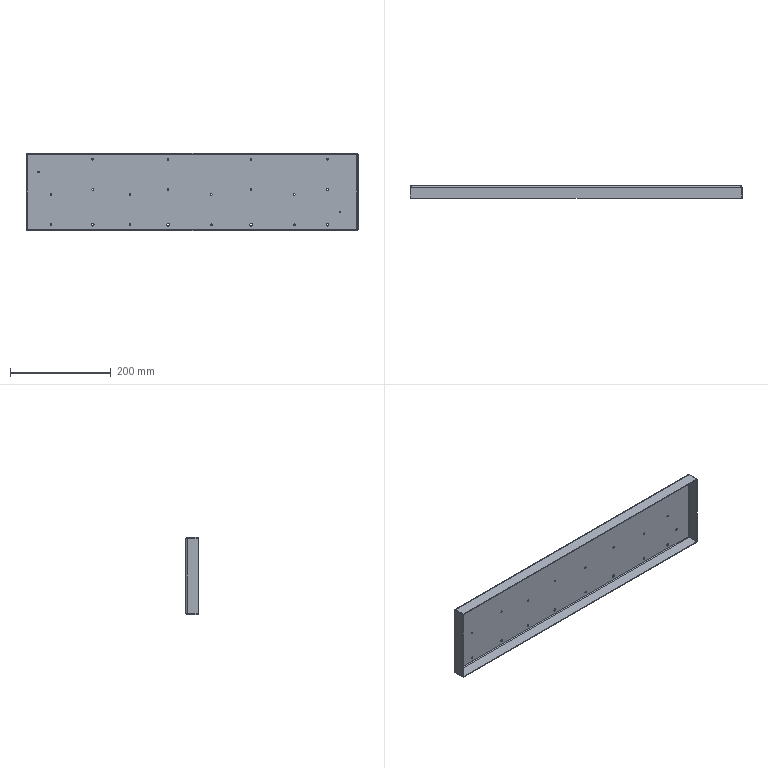Part | NX | 1 solid | 134 faces | box 660 x 25 x 154 mm | volume 219911 mm3 | cylinder 52 | cone 44 | plane 38 | commonest cylinder face diameters 3.3 x36 5.5 x8 3.2 x4 6.4 x4